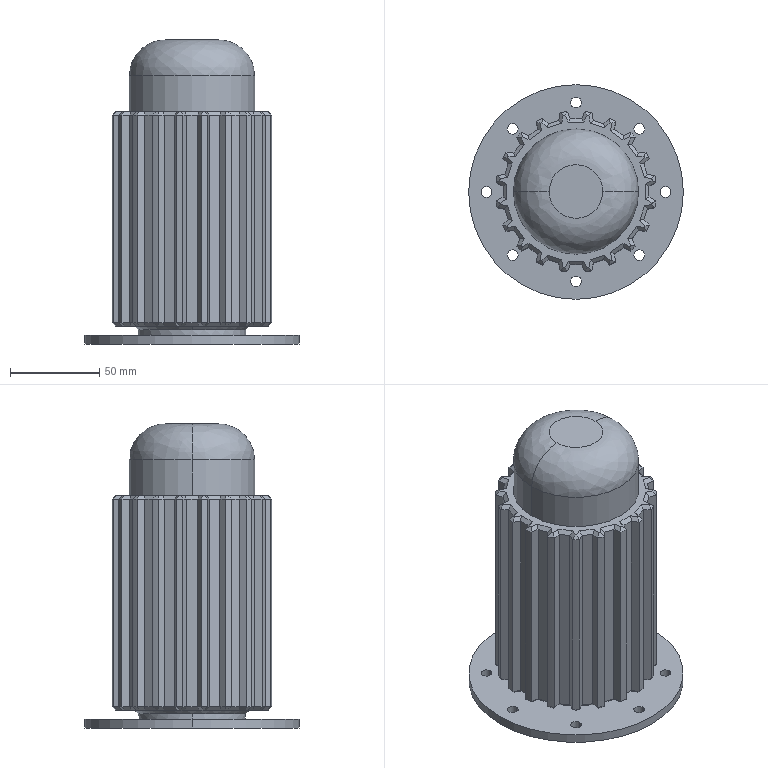Part | STEP file | Main motor | 1 solid | 271 faces | box 120 x 120 x 170 mm | volume 887990 mm3 | plane 185 | cylinder 42 | cone 42 | spline 2 | commonest cylinder face diameters 90 x20 6 x16 60 x2 70 x2 120 x2